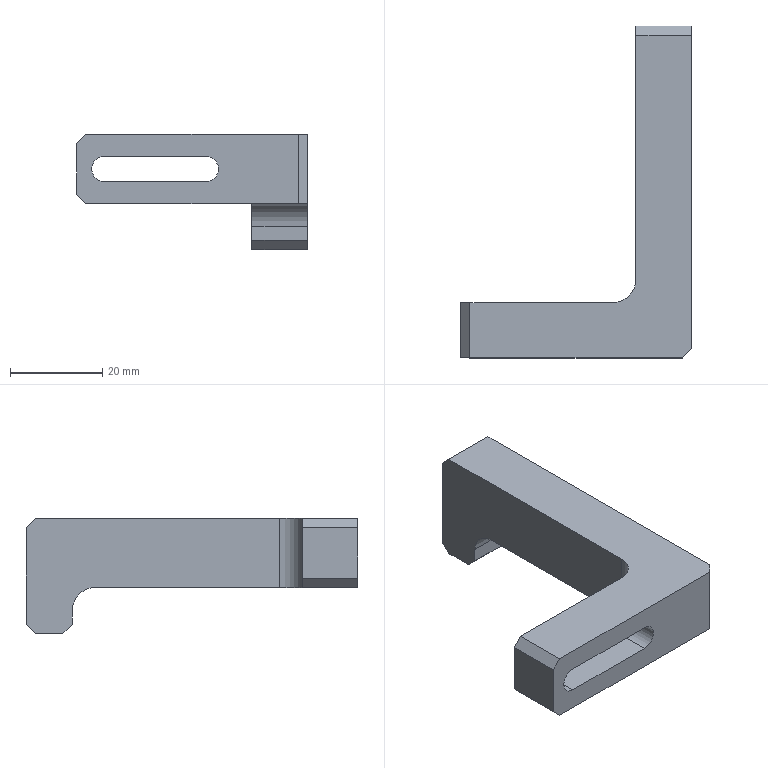NC program | NX | posted with a generic post | part box 50 x 72 x 25 mm
Lines 2586 to 2700 of 2700:
(ZLEVEL_PROFILE_COPY_1 , TOOL : D10JING)
N5170 T14 M6
N5172 G54
N5174 G17 G0 G90 X37.429 Y28.642 B0. C0. S9500 M3
N5176 G43 Z30. H14
N5178 Z1.5
N5180 G94 G1 X39.923 Y26.148 Z1.315 F1000.
N5182 X40.647 Y24.925 Z1.241
N5184 X41. Y23.549 Z1.166
N5186 Y-25.549 Z-1.407
N5188 X40.672 Y-26.864 Z-1.478
N5190 X40.004 Y-28.045 Z-1.549
N5192 X39.045 Y-29.004 Z-1.62
N5194 X37.864 Y-29.672 Z-1.691
N5196 X36.549 Y-30. Z-1.762
N5198 X23.451 Z-2.449
N5200 X22.136 Y-29.672 Z-2.52
N5202 X20.955 Y-29.004 Z-2.591
N5204 X19.996 Y-28.045 Z-2.662
N5206 X19.328 Y-26.864 Z-2.733
N5208 X19. Y-25.549 Z-2.804
N5210 Y8. Z-4.562
N5212 X-36.549 Z-7.473
N5214 X-37.864 Y8.328 Z-7.545
N5216 X-39.045 Y8.996 Z-7.616
N5218 X-40.004 Y9.955 Z-7.687
N5220 X-40.672 Y11.136 Z-7.758
N5222 X-41. Y12.451 Z-7.829
N5224 Y25.549 Z-8.515
N5226 X-40.672 Y26.864 Z-8.586
N5228 X-40.004 Y28.045 Z-8.657
N5230 X-39.045 Y29.004 Z-8.728
N5232 X-37.864 Y29.672 Z-8.8
N5234 X-36.549 Y30. Z-8.871
N5236 X34.549 Z-12.597
N5238 X35.925 Y29.647 Z-12.671
N5240 X37.148 Y28.923 Z-12.746
N5242 X39.923 Y26.148 Z-12.951
N5244 X40.647 Y24.925 Z-13.026
N5246 X41. Y23.549 Z-13.1
N5248 Y-25.549 Z-15.673
N5250 X40.672 Y-26.864 Z-15.744
N5252 X40.004 Y-28.045 Z-15.815
N5254 X39.045 Y-29.004 Z-15.887
N5256 X37.864 Y-29.672 Z-15.958
N5258 X36.549 Y-30. Z-16.029
N5260 X23.451 Z-16.715
N5262 X22.136 Y-29.672 Z-16.786
N5264 X20.955 Y-29.004 Z-16.857
N5266 X19.996 Y-28.045 Z-16.928
N5268 X19.328 Y-26.864 Z-16.999
N5270 X19. Y-25.549 Z-17.07
N5272 Y8. Z-18.829
N5274 X-36.549 Z-21.74
N5276 X-37.864 Y8.328 Z-21.811
N5278 X-39.045 Y8.996 Z-21.882
N5280 X-40.004 Y9.955 Z-21.953
N5282 X-40.672 Y11.136 Z-22.024
N5284 X-41. Y12.451 Z-22.095
N5286 Y25.549 Z-22.782
N5288 X-40.672 Y26.864 Z-22.853
N5290 X-40.004 Y28.045 Z-22.924
N5292 X-39.045 Y29.004 Z-22.995
N5294 X-37.864 Y29.672 Z-23.066
N5296 X-36.549 Y30. Z-23.137
N5298 X-1. Z-25.
N5300 X34. F1200.
N5302 G2 X37.536 Y28.536 R5.
N5304 G1 X39.536 Y26.536
N5306 G2 X41. Y23. R5.
N5308 G1 Y-25.
N5310 G2 X36. Y-30. R5.
N5312 G1 X24.
N5314 G2 X19. Y-25. R5.
N5316 G1 Y8.
N5318 X-36.
N5320 G2 X-41. Y13. R5.
N5322 G1 Y25.
N5324 G2 X-36. Y30. R5.
N5326 G1 X-1.
N5328 Z-23.5
N5330 G0 Z30.
N5332 M5
(PLANAR_MILL_COPY_COPY_COPY , TOOL : D6A45)
N5334 T01 M6
N5336 G54
N5338 G17 G0 G90 X-1.866 Y26.4 B0. C0. S9500 M3
N5340 G43 Z30. H1
N5342 Z0.5
N5344 G94 G1 Z-1. F1250.
N5346 G3 X-1. Y25.9 R1.
N5348 G1 X34.
N5350 G2 X34.636 Y25.636 R0.9
N5352 G1 X36.636 Y23.636
N5354 G2 X36.9 Y23. R0.9
N5356 G1 Y-25.
N5358 G2 X36. Y-25.9 R0.9
N5360 G1 X24.
N5362 G2 X23.1 Y-25. R0.9
N5364 G1 Y8.
N5366 G3 X19. Y12.1 R4.1
N5368 G1 X-36.
N5370 G2 X-36.9 Y13. R0.9
N5372 G1 Y25.
N5374 G2 X-36. Y25.9 R0.9
N5376 G1 X-1.
N5378 G3 X-0.134 Y26.4 R1.
N5380 G1 Z0.5
N5382 G0 Z30.
N5384 M5
N5386 M2